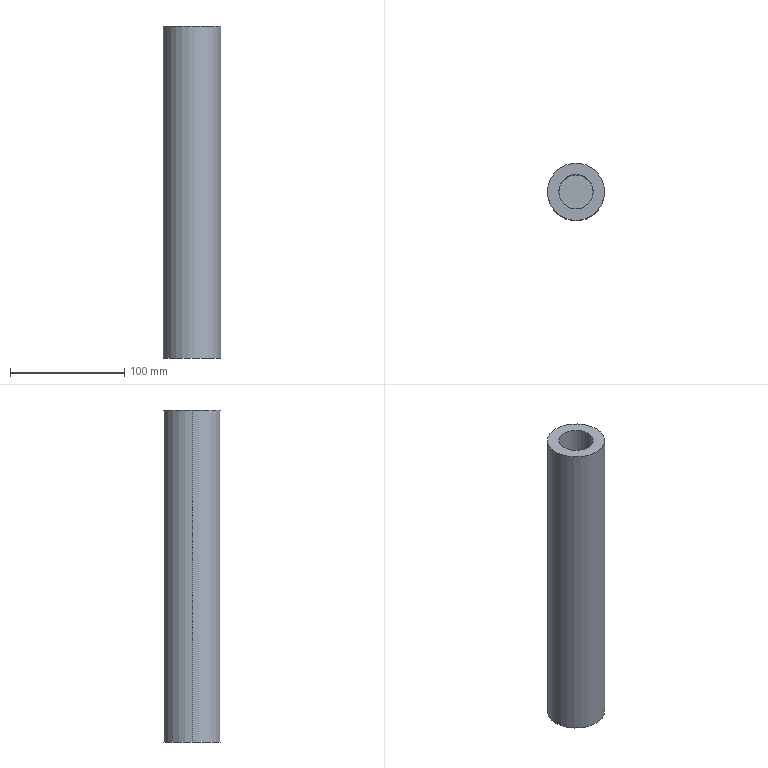Part | STEP file | Hydraulic Cylinder Rod 2 | 1 solid | 7 faces | box 50 x 50 x 290 mm | volume 385630 mm3 | cylinder 4 | plane 3 | commonest cylinder face diameters 30 x2 50 x2
STEP:
#1=CARTESIAN_POINT('',(-25.,0.,290.));
#2=VERTEX_POINT('',#1);
#3=CARTESIAN_POINT('',(25.,0.,290.));
#4=VERTEX_POINT('',#3);
#5=CARTESIAN_POINT('',(0.,0.,290.));
#6=DIRECTION('',(0.,0.,-1.));
#7=DIRECTION('',(-1.,0.,0.));
#8=AXIS2_PLACEMENT_3D('',#5,#6,#7);
#9=CIRCLE('',#8,25.);
#10=EDGE_CURVE('',#2,#4,#9,.T.);
#11=ORIENTED_EDGE('',*,*,#10,.T.);
#12=CARTESIAN_POINT('',(25.,0.,0.));
#13=VERTEX_POINT('',#12);
#14=CARTESIAN_POINT('',(25.,0.,290.));
#15=DIRECTION('',(0.,0.,-1.));
#16=VECTOR('',#15,1000.);
#17=LINE('',#14,#16);
#18=EDGE_CURVE('',#4,#13,#17,.T.);
#19=ORIENTED_EDGE('',*,*,#18,.T.);
#20=CARTESIAN_POINT('',(-25.,0.,0.));
#21=VERTEX_POINT('',#20);
#22=CARTESIAN_POINT('',(0.,0.,0.));
#23=DIRECTION('',(0.,0.,1.));
#24=DIRECTION('',(-1.,0.,0.));
#25=AXIS2_PLACEMENT_3D('',#22,#23,#24);
#26=CIRCLE('',#25,25.);
#27=EDGE_CURVE('',#13,#21,#26,.T.);
#28=ORIENTED_EDGE('',*,*,#27,.T.);
#29=CARTESIAN_POINT('',(-25.,0.,290.));
#30=DIRECTION('',(0.,0.,-1.));
#31=VECTOR('',#30,1000.);
#32=LINE('',#29,#31);
#33=EDGE_CURVE('',#2,#21,#32,.T.);
#34=ORIENTED_EDGE('',*,*,#33,.F.);
#35=EDGE_LOOP('',(#11,#19,#28,#34));
#36=FACE_OUTER_BOUND('',#35,.T.);
#37=CARTESIAN_POINT('',(0.,0.,290.));
#38=DIRECTION('',(0.,0.,-1.));
#39=DIRECTION('',(-1.,0.,0.));
#40=AXIS2_PLACEMENT_3D('',#37,#38,#39);
#41=CYLINDRICAL_SURFACE('',#40,25.);
#42=ADVANCED_FACE('',(#36),#41,.T.);
#43=CARTESIAN_POINT('',(-15.,0.,30.));
#44=VERTEX_POINT('',#43);
#45=CARTESIAN_POINT('',(15.,0.,30.));
#46=VERTEX_POINT('',#45);
#47=CARTESIAN_POINT('',(0.,0.,30.));
#48=DIRECTION('',(0.,0.,1.));
#49=DIRECTION('',(1.,0.,0.));
#50=AXIS2_PLACEMENT_3D('',#47,#48,#49);
#51=CIRCLE('',#50,15.);
#52=EDGE_CURVE('',#44,#46,#51,.T.);
#53=ORIENTED_EDGE('',*,*,#52,.F.);
#54=CARTESIAN_POINT('',(-15.,0.,290.));
#55=VERTEX_POINT('',#54);
#56=CARTESIAN_POINT('',(-15.,0.,30.));
#57=DIRECTION('',(0.,0.,1.));
#58=VECTOR('',#57,1000.);
#59=LINE('',#56,#58);
#60=EDGE_CURVE('',#44,#55,#59,.T.);
#61=ORIENTED_EDGE('',*,*,#60,.T.);
#62=CARTESIAN_POINT('',(15.,0.,290.));
#63=VERTEX_POINT('',#62);
#64=CARTESIAN_POINT('',(0.,0.,290.));
#65=DIRECTION('',(0.,0.,-1.));
#66=DIRECTION('',(1.,0.,0.));
#67=AXIS2_PLACEMENT_3D('',#64,#65,#66);
#68=CIRCLE('',#67,15.);
#69=EDGE_CURVE('',#63,#55,#68,.T.);
#70=ORIENTED_EDGE('',*,*,#69,.F.);
#71=CARTESIAN_POINT('',(15.,0.,30.));
#72=DIRECTION('',(0.,0.,1.));
#73=VECTOR('',#72,1000.);
#74=LINE('',#71,#73);
#75=EDGE_CURVE('',#46,#63,#74,.T.);
#76=ORIENTED_EDGE('',*,*,#75,.F.);
#77=EDGE_LOOP('',(#53,#61,#70,#76));
#78=FACE_OUTER_BOUND('',#77,.T.);
#79=CARTESIAN_POINT('',(0.,0.,30.));
#80=DIRECTION('',(0.,0.,1.));
#81=DIRECTION('',(1.,0.,0.));
#82=AXIS2_PLACEMENT_3D('',#79,#80,#81);
#83=CYLINDRICAL_SURFACE('',#82,15.);
#84=ADVANCED_FACE('',(#78),#83,.F.);
#85=ORIENTED_EDGE('',*,*,#18,.F.);
#86=CARTESIAN_POINT('',(0.,0.,290.));
#87=DIRECTION('',(0.,0.,-1.));
#88=DIRECTION('',(-1.,0.,0.));
#89=AXIS2_PLACEMENT_3D('',#86,#87,#88);
#90=CIRCLE('',#89,25.);
#91=EDGE_CURVE('',#4,#2,#90,.T.);
#92=ORIENTED_EDGE('',*,*,#91,.T.);
#93=ORIENTED_EDGE('',*,*,#33,.T.);
#94=CARTESIAN_POINT('',(0.,0.,0.));
#95=DIRECTION('',(0.,0.,1.));
#96=DIRECTION('',(-1.,0.,0.));
#97=AXIS2_PLACEMENT_3D('',#94,#95,#96);
#98=CIRCLE('',#97,25.);
#99=EDGE_CURVE('',#21,#13,#98,.T.);
#100=ORIENTED_EDGE('',*,*,#99,.T.);
#101=EDGE_LOOP('',(#85,#92,#93,#100));
#102=FACE_OUTER_BOUND('',#101,.T.);
#103=CARTESIAN_POINT('',(0.,0.,290.));
#104=DIRECTION('',(0.,0.,-1.));
#105=DIRECTION('',(-1.,0.,0.));
#106=AXIS2_PLACEMENT_3D('',#103,#104,#105);
#107=CYLINDRICAL_SURFACE('',#106,25.);
#108=ADVANCED_FACE('',(#102),#107,.T.);
#109=ORIENTED_EDGE('',*,*,#99,.F.);
#110=ORIENTED_EDGE('',*,*,#27,.F.);
#111=EDGE_LOOP('',(#109,#110));
#112=FACE_OUTER_BOUND('',#111,.T.);
#113=CARTESIAN_POINT('',(0.,0.,0.));
#114=DIRECTION('',(0.,0.,1.));
#115=DIRECTION('',(1.,0.,0.));
#116=AXIS2_PLACEMENT_3D('',#113,#114,#115);
#117=PLANE('',#116);
#118=ADVANCED_FACE('',(#112),#117,.F.);
#119=ORIENTED_EDGE('',*,*,#10,.F.);
#120=ORIENTED_EDGE('',*,*,#91,.F.);
#121=EDGE_LOOP('',(#119,#120));
#122=FACE_OUTER_BOUND('',#121,.T.);
#123=ORIENTED_EDGE('',*,*,#69,.T.);
#124=CARTESIAN_POINT('',(0.,0.,290.));
#125=DIRECTION('',(0.,0.,-1.));
#126=DIRECTION('',(1.,0.,0.));
#127=AXIS2_PLACEMENT_3D('',#124,#125,#126);
#128=CIRCLE('',#127,15.);
#129=EDGE_CURVE('',#55,#63,#128,.T.);
#130=ORIENTED_EDGE('',*,*,#129,.T.);
#131=EDGE_LOOP('',(#123,#130));
#132=FACE_BOUND('',#131,.T.);
#133=CARTESIAN_POINT('',(0.,0.,290.));
#134=DIRECTION('',(0.,0.,1.));
#135=DIRECTION('',(1.,0.,0.));
#136=AXIS2_PLACEMENT_3D('',#133,#134,#135);
#137=PLANE('',#136);
#138=ADVANCED_FACE('',(#122,#132),#137,.T.);
#139=ORIENTED_EDGE('',*,*,#60,.F.);
#140=CARTESIAN_POINT('',(0.,0.,30.));
#141=DIRECTION('',(0.,0.,1.));
#142=DIRECTION('',(1.,0.,0.));
#143=AXIS2_PLACEMENT_3D('',#140,#141,#142);
#144=CIRCLE('',#143,15.);
#145=EDGE_CURVE('',#46,#44,#144,.T.);
#146=ORIENTED_EDGE('',*,*,#145,.F.);
#147=ORIENTED_EDGE('',*,*,#75,.T.);
#148=ORIENTED_EDGE('',*,*,#129,.F.);
#149=EDGE_LOOP('',(#139,#146,#147,#148));
#150=FACE_OUTER_BOUND('',#149,.T.);
#151=CARTESIAN_POINT('',(0.,0.,30.));
#152=DIRECTION('',(0.,0.,1.));
#153=DIRECTION('',(1.,0.,0.));
#154=AXIS2_PLACEMENT_3D('',#151,#152,#153);
#155=CYLINDRICAL_SURFACE('',#154,15.);
#156=ADVANCED_FACE('',(#150),#155,.F.);
#157=ORIENTED_EDGE('',*,*,#145,.T.);
#158=ORIENTED_EDGE('',*,*,#52,.T.);
#159=EDGE_LOOP('',(#157,#158));
#160=FACE_OUTER_BOUND('',#159,.T.);
#161=CARTESIAN_POINT('',(0.,0.,30.));
#162=DIRECTION('',(0.,0.,1.));
#163=DIRECTION('',(1.,0.,0.));
#164=AXIS2_PLACEMENT_3D('',#161,#162,#163);
#165=PLANE('',#164);
#166=ADVANCED_FACE('',(#160),#165,.T.);
#167=CLOSED_SHELL('',(#42,#84,#108,#118,#138,#156,#166));
#168=MANIFOLD_SOLID_BREP('',#167);
#169=CARTESIAN_POINT('',(0.,0.,0.));
#170=DIRECTION('',(0.,0.,1.));
#171=DIRECTION('',(1.,0.,0.));
#172=AXIS2_PLACEMENT_3D('',#169,#170,#171);
#173=(LENGTH_UNIT()NAMED_UNIT(*)SI_UNIT(.MILLI.,.METRE.));
#174=UNCERTAINTY_MEASURE_WITH_UNIT(LENGTH_MEASURE(0.00001),#173,'','');
#175=(NAMED_UNIT(*)PLANE_ANGLE_UNIT()SI_UNIT($,.RADIAN.));
#176=(NAMED_UNIT(*)SI_UNIT($,.STERADIAN.)SOLID_ANGLE_UNIT());
#177=(GEOMETRIC_REPRESENTATION_CONTEXT(3)GLOBAL_UNCERTAINTY_ASSIGNED_CONTEXT((#174))GLOBAL_UNIT_ASSIGNED_CONTEXT((#173,#175,#176))REPRESENTATION_CONTEXT('',''));
#178=ADVANCED_BREP_SHAPE_REPRESENTATION('',(#168,#172),#177);